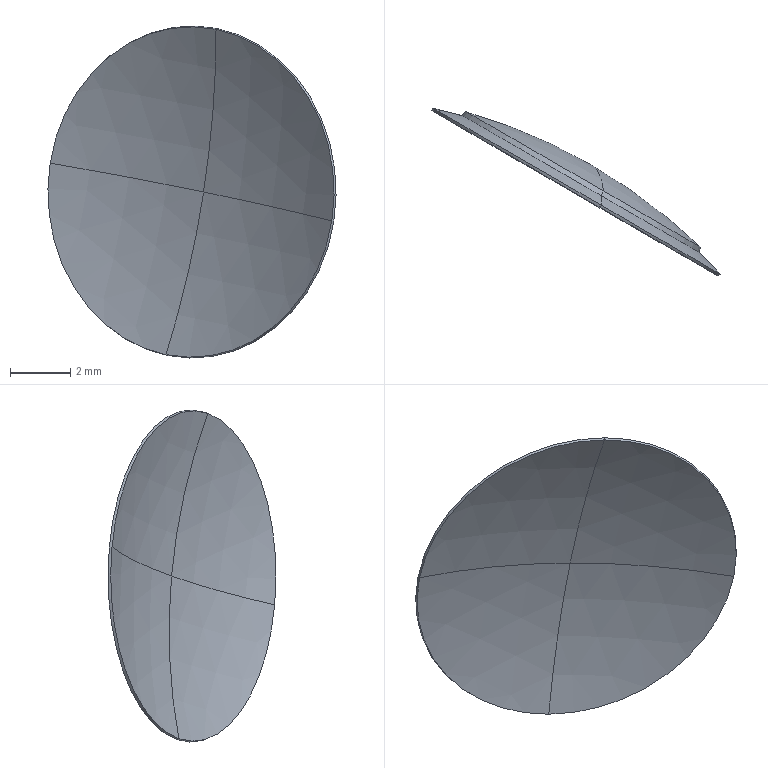Part | SolidWorks | features BaseBody 1 | 1 solid | 16 faces | box 9.592 x 5.588 x 11.054 mm | volume 19.29 mm3 | sphere 12 | cone 4